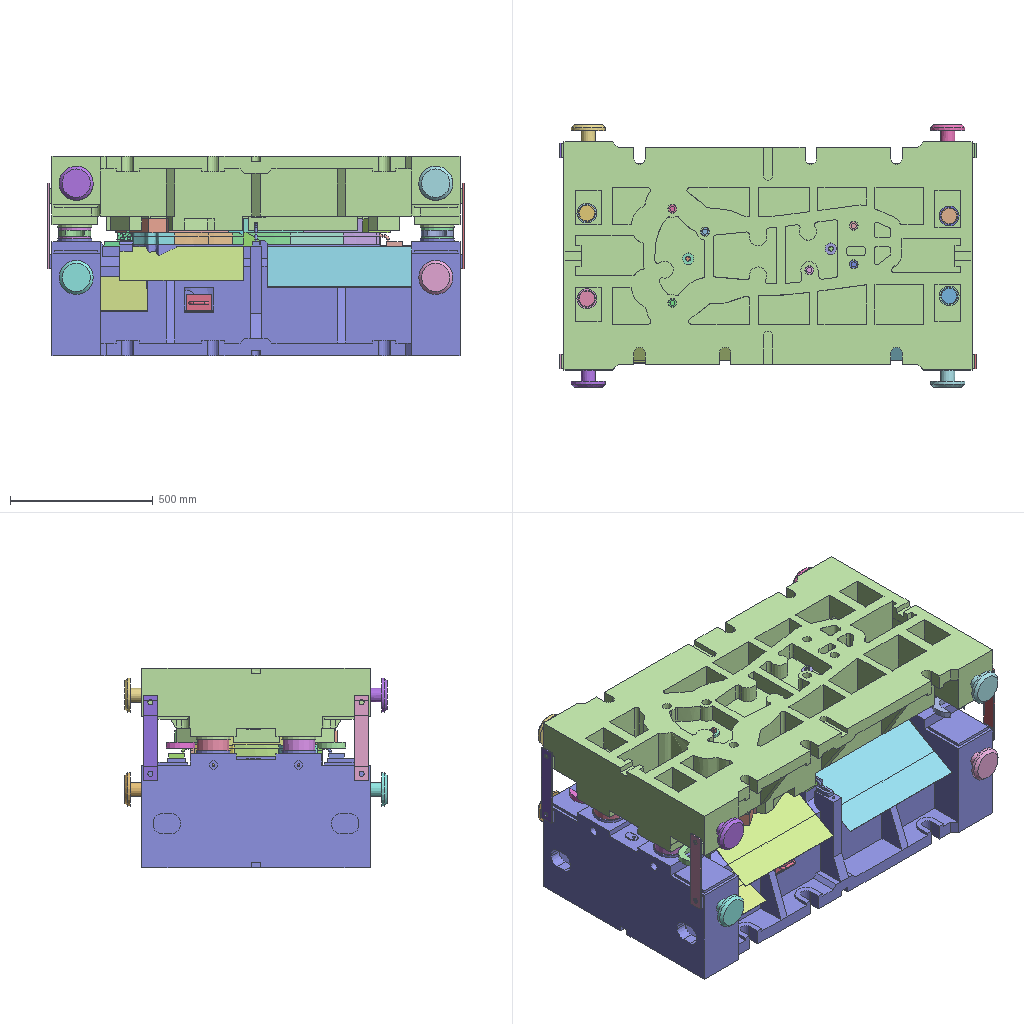Assembly | NX | 136 different items | 136 placed | box 1460 x 920 x 700 mm
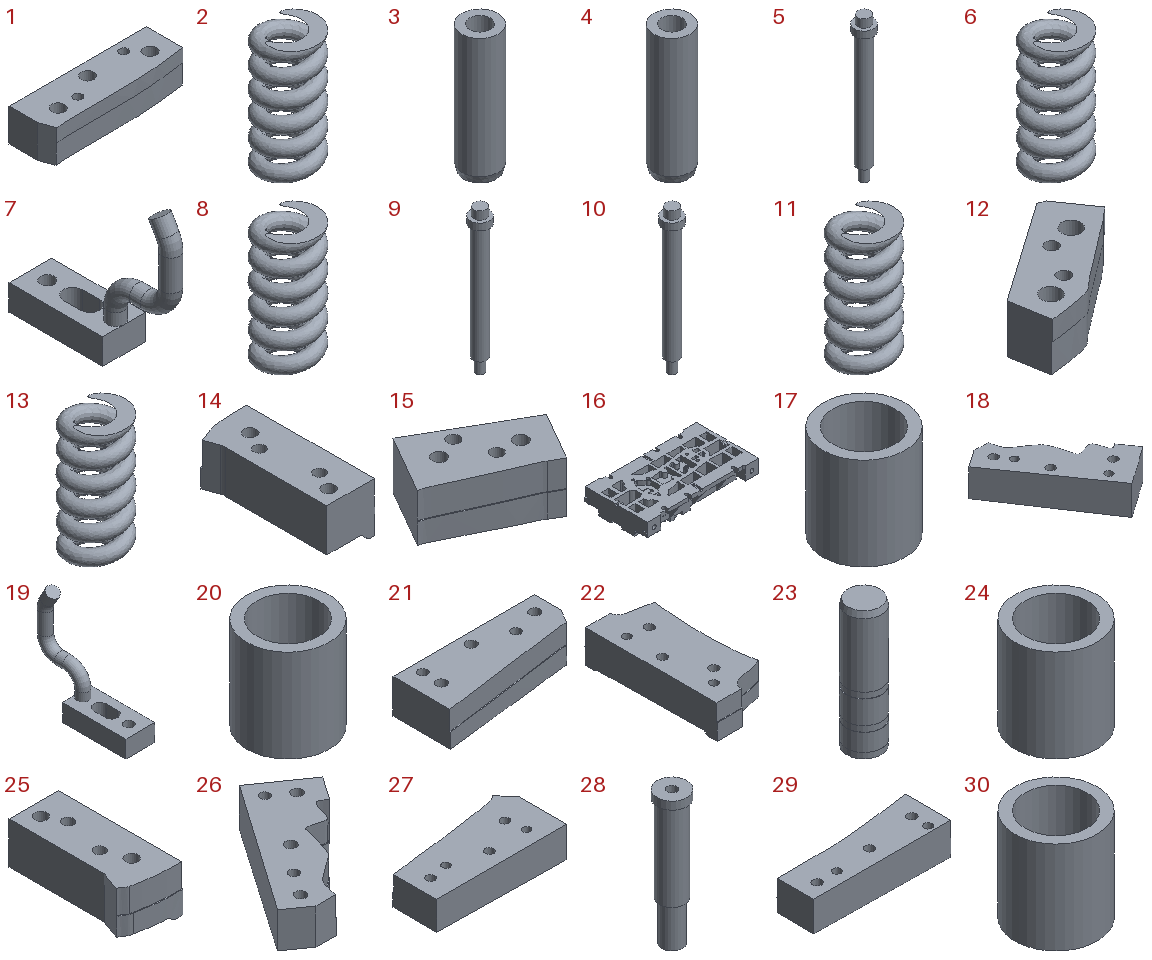Parts list (item | quantity | size | volume | features):
1 | x1 | 210 x 65.035 x 50 mm | 599667 mm3 | features solid 2
2 | x1 | 48.883 x 48.763 x 105 mm | 73970 mm3 | features solid 2
3 | x1 | 23 x 23 x 80 mm | 22449 mm3 | features solid 2
4 | x1 | 23 x 23 x 80 mm | 22449 mm3 | features solid 2
5 | x1 | 28 x 28 x 212 mm | 64862 mm3 | features solid 2
6 | x1 | 48.883 x 48.763 x 105 mm | 73970 mm3 | features solid 2
7 | x1 | 25 x 87.5 x 83.84 mm | 23805 mm3 | features solid 2
8 | x1 | 48.883 x 48.763 x 105 mm | 73970 mm3 | features solid 2
9 | x1 | 28 x 28 x 212 mm | 64862 mm3 | features solid 2
10 | x1 | 28 x 28 x 212 mm | 64862 mm3 | features solid 2
11 | x1 | 48.883 x 48.763 x 105 mm | 73970 mm3 | features solid 2
12 | x1 | 134.129 x 111.662 x 50 mm | 319985 mm3 | features solid 2
13 | x1 | 48.883 x 48.763 x 105 mm | 73970 mm3 | features solid 2
14 | x1 | 58.448 x 138.583 x 54 mm | 307683 mm3 | features solid 2
15 | x1 | 128.226 x 102.703 x 49 mm | 276802 mm3 | features solid 2
16 | x1 | 1450 x 800 x 260 mm | 132746241 mm3 | features solid 2
17 | x1 | 80 x 80 x 90 mm | 197920 mm3 | features solid 2
18 | x1 | 174.157 x 178.927 x 49.162 mm | 505819 mm3 | features solid 2
19 | x1 | 25 x 87.5 x 83.84 mm | 23805 mm3 | features solid 2
20 | x1 | 80 x 80 x 90 mm | 197920 mm3 | features solid 2
21 | x1 | 190 x 77.202 x 49 mm | 533437 mm3 | features solid 2
22 | x1 | 90.456 x 205 x 51 mm | 693482 mm3 | features solid 2
23 | x1 | 60 x 60 x 220 mm | 616781 mm3 | features solid 2
24 | x1 | 80 x 80 x 90 mm | 197920 mm3 | features solid 2
25 | x1 | 62.75 x 136.771 x 54 mm | 322596 mm3 | features solid 2
26 | x1 | 178.021 x 184.327 x 49 mm | 541406 mm3 | features solid 2
27 | x1 | 210 x 100.542 x 49 mm | 790054 mm3 | features solid 2
28 | x1 | 19 x 19 x 85 mm | 15462 mm3 | features solid 2
29 | x1 | 210 x 70.368 x 49 mm | 559082 mm3 | features solid 2
30 | x1 | 80 x 80 x 90 mm | 197920 mm3 | features solid 2
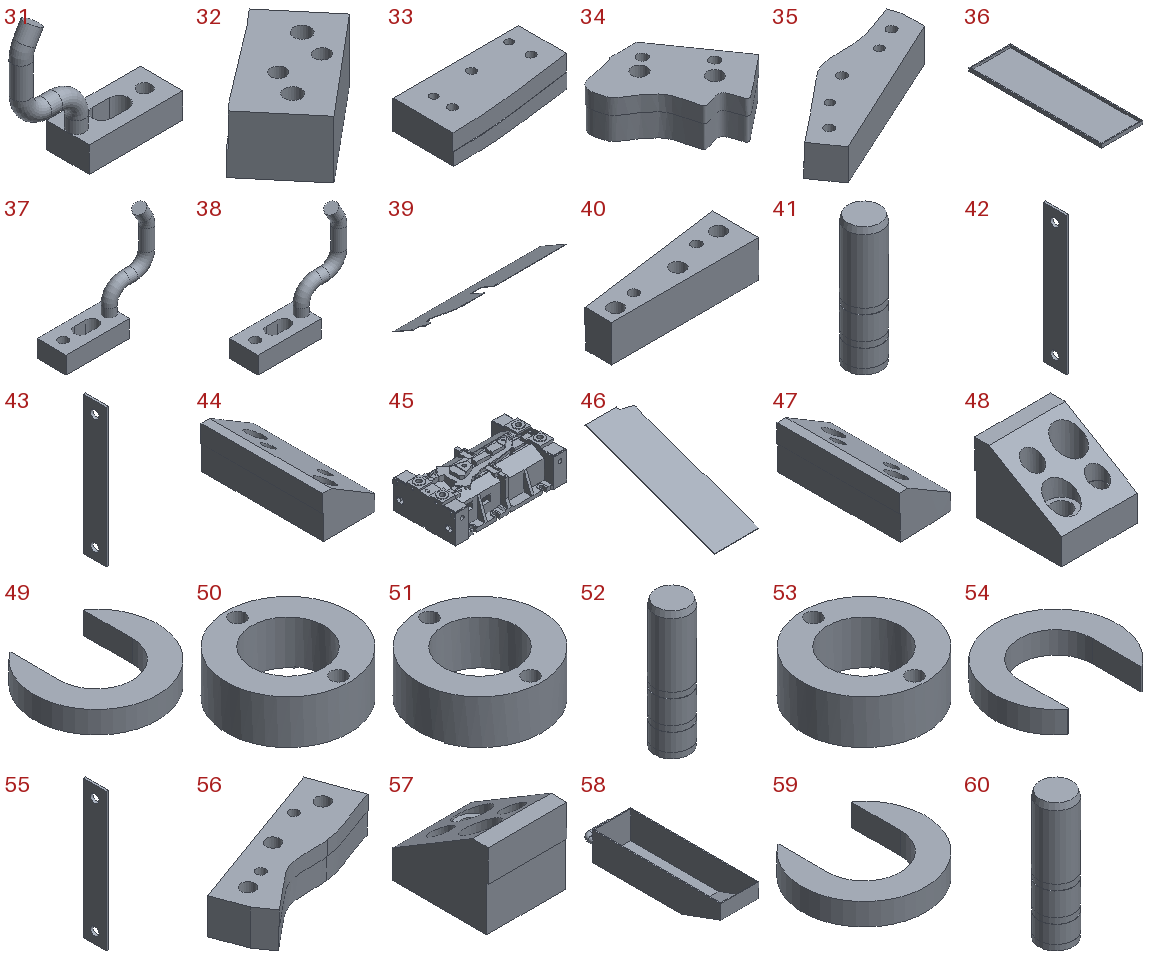31 | x1 | 87.5 x 25 x 83.84 mm | 23805 mm3 | features solid 2
32 | x1 | 115.597 x 108.38 x 49 mm | 247805 mm3 | features solid 2
33 | x1 | 200 x 96.579 x 49 mm | 800737 mm3 | features solid 2
34 | x1 | 150.505 x 135.487 x 50 mm | 528166 mm3 | features solid 2
35 | x1 | 236.188 x 148.081 x 48.904 mm | 669282 mm3 | features solid 2
36 | x1 | 86 x 276 x 7 mm | 54632 mm3 | features solid 2
37 | x1 | 87.5 x 25 x 83.84 mm | 23805 mm3 | features solid 2
38 | x1 | 87.5 x 25 x 83.84 mm | 23805 mm3 | features solid 2
39 | x1 | 1023 x 199.923 x 116.58 mm | 412824 mm3 | features solid 2
40 | x1 | 200 x 62.717 x 50 mm | 447168 mm3 | features solid 2
41 | x1 | 60 x 60 x 220 mm | 616781 mm3 | features solid 2
42 | x1 | 5 x 50 x 300 mm | 72455 mm3 | features solid 2
43 | x1 | 5 x 50 x 300 mm | 72455 mm3 | features solid 2
44 | x1 | 60 x 138.619 x 48 mm | 266827 mm3 | features solid 2
45 | x1 | 1450 x 800 x 440 mm | 184592094 mm3 | features solid 2
46 | x1 | 165 x 478.472 x 175.78 mm | 163563 mm3 | features solid 2
47 | x1 | 60 x 136.579 x 48 mm | 262854 mm3 | features solid 2
48 | x1 | 52.578 x 60 x 48 mm | 89054 mm3 | features solid 2
49 | x1 | 112 x 100.638 x 20 mm | 93427 mm3 | features solid 2
50 | x1 | 112 x 112 x 40 mm | 247574 mm3 | features solid 2
51 | x1 | 112 x 112 x 40 mm | 247574 mm3 | features solid 2
52 | x1 | 60 x 60 x 220 mm | 616781 mm3 | features solid 2
53 | x1 | 112 x 112 x 40 mm | 247574 mm3 | features solid 2
54 | x1 | 112 x 100.638 x 20 mm | 93427 mm3 | features solid 2
55 | x1 | 5 x 50 x 300 mm | 72455 mm3 | features solid 2
56 | x1 | 235.557 x 144.564 x 50 mm | 672239 mm3 | features solid 2
57 | x1 | 49.578 x 60 x 48 mm | 81453 mm3 | features solid 2
58 | x1 | 80 x 300 x 60 mm | 122773 mm3 | features solid 2
59 | x1 | 112 x 100.638 x 20 mm | 93427 mm3 | features solid 2
60 | x1 | 60 x 60 x 220 mm | 616781 mm3 | features solid 2
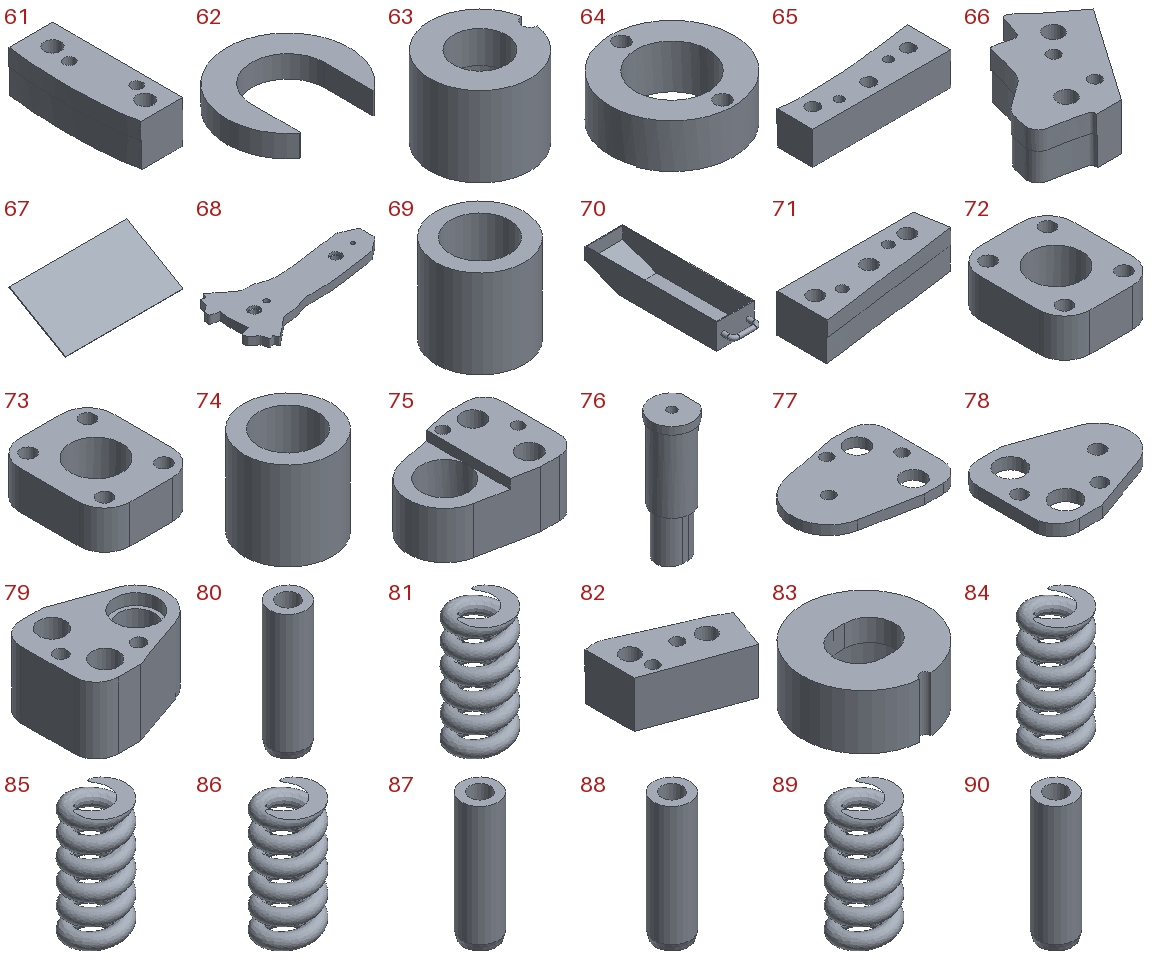61 | x1 | 56.479 x 155 x 50 mm | 388259 mm3 | features solid 2
62 | x1 | 112 x 100.638 x 20 mm | 93427 mm3 | features solid 2
63 | x1 | 24.84 x 25 x 20 mm | 6021 mm3 | features solid 2
64 | x1 | 112 x 112 x 40 mm | 247574 mm3 | features solid 2
65 | x1 | 210 x 66.209 x 50 mm | 539295 mm3 | features solid 2
66 | x1 | 144.972 x 140.193 x 50 mm | 503564 mm3 | features solid 2
67 | x1 | 505 x 243.026 x 141.466 mm | 282262 mm3 | features solid 2
68 | x1 | 860.43 x 430.677 x 45 mm | 8766839 mm3 | features solid 2
69 | x1 | 60 x 60 x 60 mm | 94248 mm3 | features solid 2
70 | x1 | 90 x 345 x 60 mm | 148544 mm3 | features solid 2
71 | x1 | 185.528 x 65.269 x 50 mm | 442182 mm3 | features solid 2
72 | x1 | 110 x 130 x 45 mm | 451871 mm3 | features solid 2
73 | x1 | 110 x 130 x 45 mm | 451871 mm3 | features solid 2
74 | x1 | 60 x 60 x 60 mm | 94248 mm3 | features solid 2
75 | x1 | 65.5 x 50 x 30 mm | 51666 mm3 | features solid 2
76 | x1 | 26.5 x 28 x 85 mm | 36969 mm3 | features solid 2
77 | x1 | 65.5 x 50 x 5 mm | 12017 mm3 | features solid 2
78 | x1 | 54 x 44 x 5 mm | 7831 mm3 | features solid 2
79 | x1 | 54 x 44 x 30 mm | 37935 mm3 | features solid 2
80 | x1 | 23 x 23 x 80 mm | 22449 mm3 | features solid 2
81 | x1 | 48.883 x 48.763 x 105 mm | 73970 mm3 | features solid 2
82 | x1 | 115.07 x 90.062 x 50 mm | 264486 mm3 | features solid 2
83 | x1 | 45 x 44.911 x 20 mm | 16859 mm3 | features solid 2
84 | x1 | 48.883 x 48.763 x 105 mm | 73970 mm3 | features solid 2
85 | x1 | 48.883 x 48.763 x 105 mm | 73970 mm3 | features solid 2
86 | x1 | 48.883 x 48.763 x 105 mm | 73970 mm3 | features solid 2
87 | x1 | 23 x 23 x 80 mm | 22449 mm3 | features solid 2
88 | x1 | 23 x 23 x 80 mm | 22449 mm3 | features solid 2
89 | x1 | 48.883 x 48.763 x 105 mm | 73970 mm3 | features solid 2
90 | x1 | 23 x 23 x 80 mm | 22449 mm3 | features solid 2
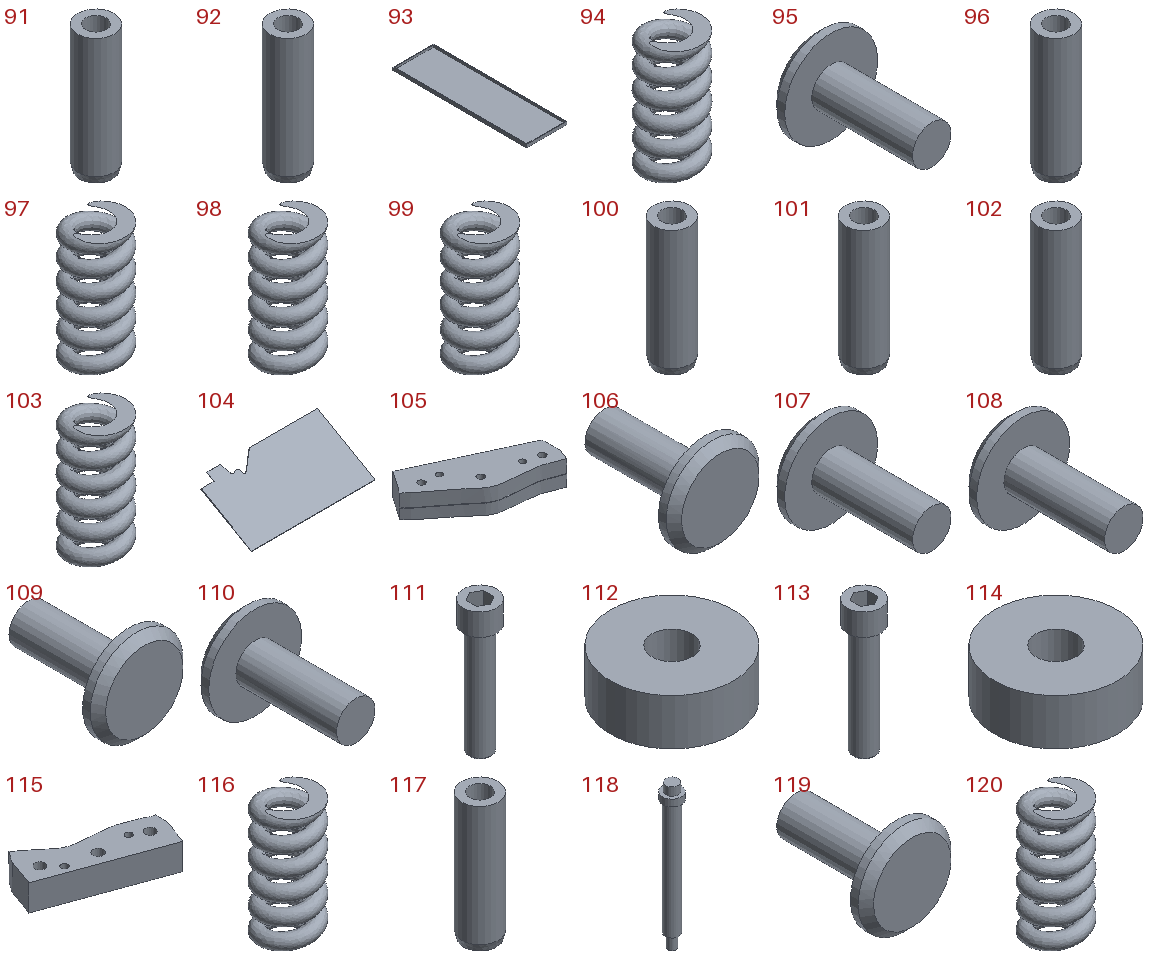91 | x1 | 23 x 23 x 80 mm | 22449 mm3 | features solid 2
92 | x1 | 23 x 23 x 80 mm | 22449 mm3 | features solid 2
93 | x1 | 96 x 321 x 7 mm | 69892 mm3 | features solid 2
94 | x1 | 48.883 x 48.763 x 105 mm | 73970 mm3 | features solid 2
95 | x1 | 120 x 150 x 120 mm | 463647 mm3 | features solid 2
96 | x1 | 23 x 23 x 80 mm | 22449 mm3 | features solid 2
97 | x1 | 48.883 x 48.763 x 105 mm | 73970 mm3 | features solid 2
98 | x1 | 48.883 x 48.763 x 105 mm | 73970 mm3 | features solid 2
99 | x1 | 48.883 x 48.763 x 105 mm | 73970 mm3 | features solid 2
100 | x1 | 23 x 23 x 80 mm | 22449 mm3 | features solid 2
101 | x1 | 23 x 23 x 80 mm | 22449 mm3 | features solid 2
102 | x1 | 23 x 23 x 80 mm | 22449 mm3 | features solid 2
103 | x1 | 48.883 x 48.763 x 105 mm | 73970 mm3 | features solid 2
104 | x1 | 433.5 x 203.038 x 118.379 mm | 193522 mm3 | features solid 2
105 | x1 | 234.961 x 152.688 x 48.86 mm | 747452 mm3 | features solid 2
106 | x1 | 120 x 150 x 120 mm | 463647 mm3 | features solid 2
107 | x1 | 120 x 150 x 120 mm | 463647 mm3 | features solid 2
108 | x1 | 120 x 150 x 120 mm | 463647 mm3 | features solid 2
109 | x1 | 120 x 150 x 120 mm | 463647 mm3 | features solid 2
110 | x1 | 120 x 150 x 120 mm | 463647 mm3 | features solid 2
111 | x1 | 18 x 18 x 72 mm | 9247 mm3 | features solid 2
112 | x1 | 40 x 40 x 15 mm | 16859 mm3 | features solid 2
113 | x1 | 18 x 18 x 72 mm | 9247 mm3 | features solid 2
114 | x1 | 40 x 40 x 15 mm | 16859 mm3 | features solid 2
115 | x1 | 233.69 x 149.736 x 50 mm | 721253 mm3 | features solid 2
116 | x1 | 48.883 x 48.763 x 105 mm | 73970 mm3 | features solid 2
117 | x1 | 23 x 23 x 80 mm | 22449 mm3 | features solid 2
118 | x1 | 28 x 28 x 212 mm | 64862 mm3 | features solid 2
119 | x1 | 120 x 150 x 120 mm | 463647 mm3 | features solid 2
120 | x1 | 48.883 x 48.763 x 105 mm | 73970 mm3 | features solid 2
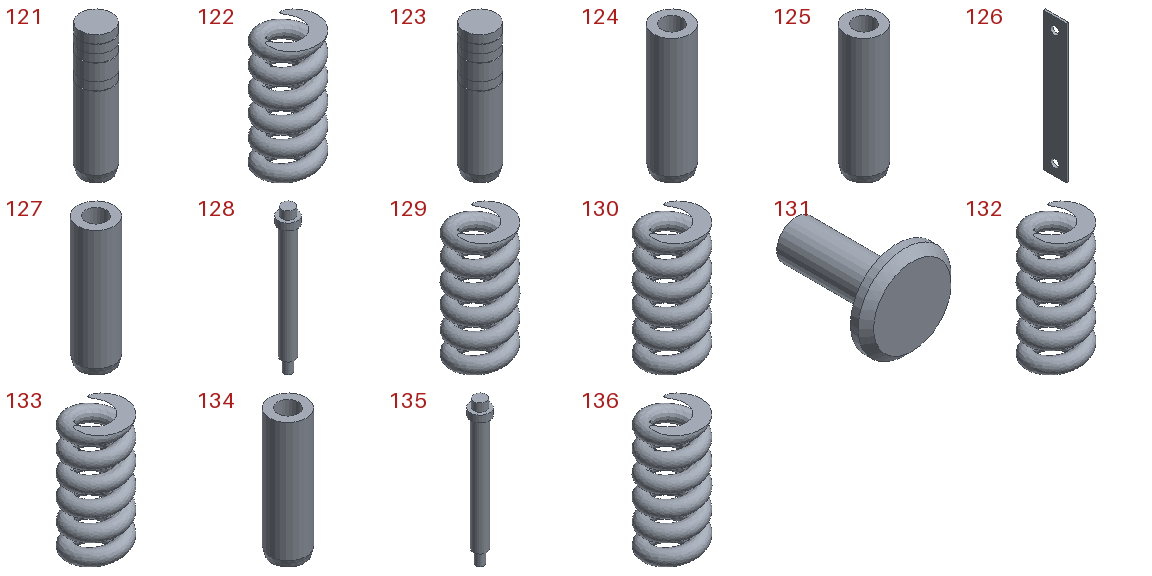121 | x1 | 40 x 40 x 160 mm | 197592 mm3 | features solid 2
122 | x1 | 48.883 x 48.763 x 105 mm | 73970 mm3 | features solid 2
123 | x1 | 40 x 40 x 160 mm | 197592 mm3 | features solid 2
124 | x1 | 23 x 23 x 80 mm | 22449 mm3 | features solid 2
125 | x1 | 23 x 23 x 80 mm | 22449 mm3 | features solid 2
126 | x1 | 5 x 50 x 300 mm | 72455 mm3 | features solid 2
127 | x1 | 23 x 23 x 80 mm | 22449 mm3 | features solid 2
128 | x1 | 28 x 28 x 212 mm | 64862 mm3 | features solid 2
129 | x1 | 48.883 x 48.763 x 105 mm | 73970 mm3 | features solid 2
130 | x1 | 48.883 x 48.763 x 105 mm | 73970 mm3 | features solid 2
131 | x1 | 120 x 150 x 120 mm | 463647 mm3 | features solid 2
132 | x1 | 48.883 x 48.763 x 105 mm | 73970 mm3 | features solid 2
133 | x1 | 48.883 x 48.763 x 105 mm | 73970 mm3 | features solid 2
134 | x1 | 23 x 23 x 80 mm | 22449 mm3 | features solid 2
135 | x1 | 28 x 28 x 212 mm | 64862 mm3 | features solid 2
136 | x1 | 48.883 x 48.763 x 105 mm | 73970 mm3 | features solid 2